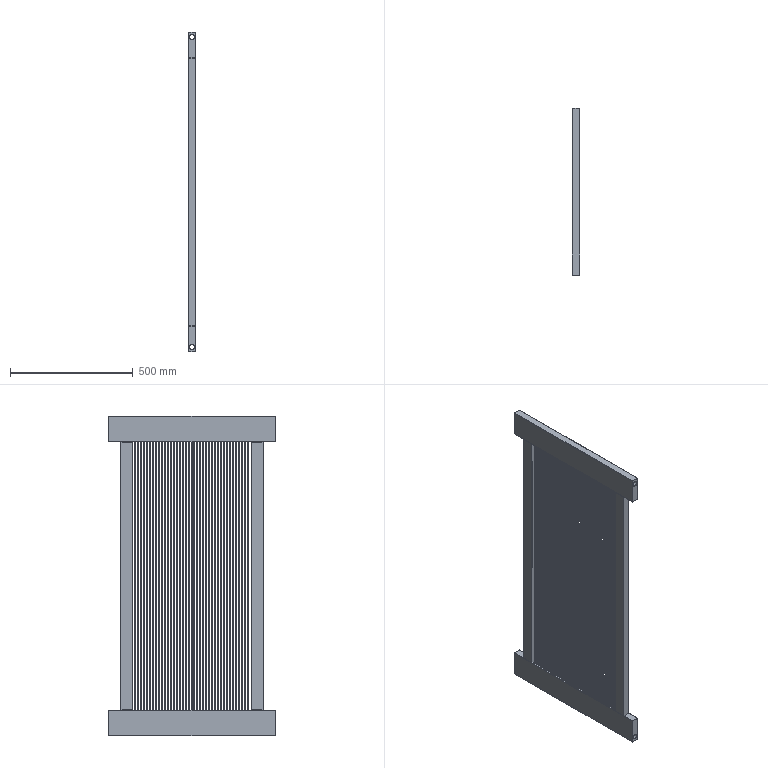Part | SolidWorks | features Fillet 4, ICE 3, Extrusion 1 | 84 solids | 422 faces | box 30 x 680 x 1300 mm | volume 7397272 mm3 | cylinder 208 | plane 184 | sphere 24 | torus 6 | commonest cylinder face diameters 2 x204 20 x4